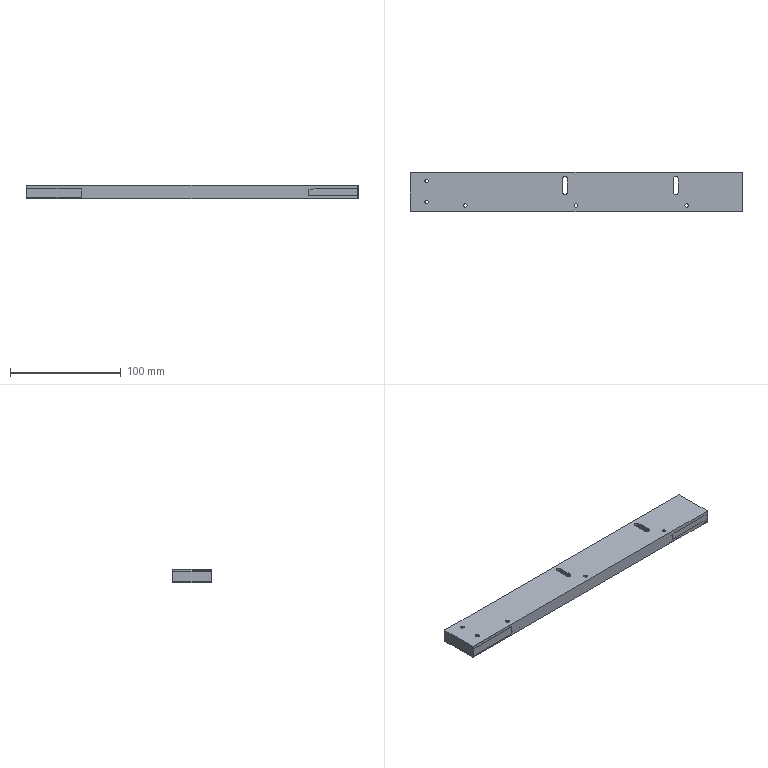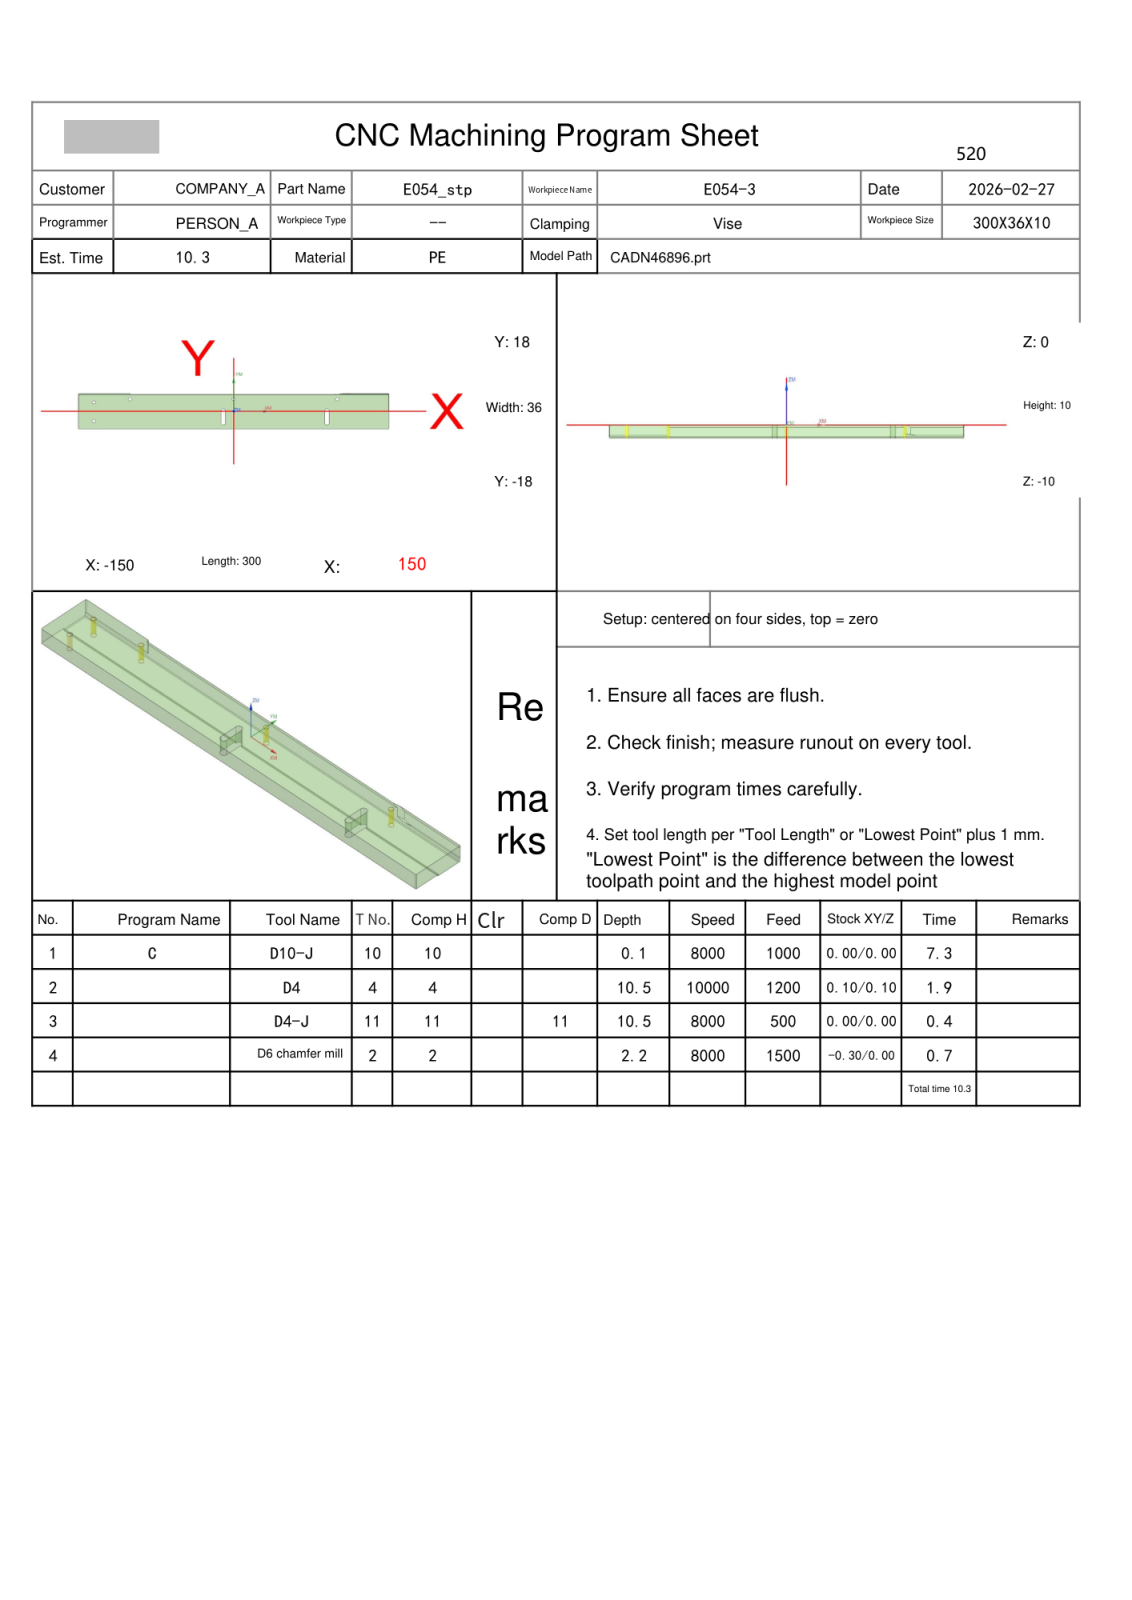NC program | NX | posted by the shop | part box 300 x 36 x 12 mm
Whole program:
%
O0001
(Machine time: 11.00 MIN)
(===Total Tool:4===)
(T10=D10-J  D=10.  R=0.   D-  H10 Z=0.    )
(T4=D4      D=4.   R=0.   D-  H04 Z=-10.5 )
(T11=D4-J   D=4.   R=0.   D11 H11 Z=-10.5 )
(T2=D6 chamfer mill   D=6.   R=0.   D-  H02 Z=-2.17 )
G80 G90 G17 G49 G40
G91 G28 Z0
M01
N1 T10 M06
(D10-J  D=10. R=0. H=10 ce=0.00 di=0.10)
G00 G90 G54 X-167. Y1.111 M03 S8000
G43 H10 Z50.
M08
Z2.55
G01 Z.55 F1000.
X-155. Y13.111
X-145.111 Y23.
X-135.222
X-155. Y3.222
Y-6.667
X-125.333 Y23.
X-115.444
X-155. Y-16.556
Y-23.
X-151.556
X-105.556 Y23.
X-95.667
X-141.667 Y-23.
X-131.778
X-85.778 Y23.
X-75.889
X-121.889 Y-23.
X-112.
X-66. Y23.
X-56.111
X-102.111 Y-23.
X-92.222
X-46.222 Y23.
X-36.333
X-82.333 Y-23.
X-72.444
X-26.444 Y23.
X-16.556
X-62.556 Y-23.
X-52.667
X-6.667 Y23.
X3.222
X-42.778 Y-23.
X-32.889
X13.111 Y23.
X23.
X-23. Y-23.
X-13.111
X32.889 Y23.
X42.778
X-3.222 Y-23.
X6.667
X52.667 Y23.
X62.556
X16.556 Y-23.
X26.444
X72.444 Y23.
X82.333
X36.333 Y-23.
X46.222
X92.222 Y23.
X102.111
X56.111 Y-23.
X66.
X112. Y23.
X121.889
X75.889 Y-23.
X85.778
X131.778 Y23.
X141.667
X95.667 Y-23.
X105.556
X151.556 Y23.
X155.
Y16.556
X115.444 Y-23.
X125.333
X155. Y6.667
Y-3.222
X135.222 Y-23.
X145.111
X155. Y-13.111
X167. Y-1.111
Z2.55
G00 Z4.
X-167. Y1.111
Z2.1
G01 Z.1
X-155. Y13.111
X-145.111 Y23.
X-135.222
X-155. Y3.222
Y-6.667
X-125.333 Y23.
X-115.444
X-155. Y-16.556
Y-23.
X-151.556
X-105.556 Y23.
X-95.667
X-141.667 Y-23.
X-131.778
X-85.778 Y23.
X-75.889
X-121.889 Y-23.
X-112.
X-66. Y23.
X-56.111
X-102.111 Y-23.
X-92.222
X-46.222 Y23.
X-36.333
X-82.333 Y-23.
X-72.444
X-26.444 Y23.
X-16.556
X-62.556 Y-23.
X-52.667
X-6.667 Y23.
X3.222
X-42.778 Y-23.
X-32.889
X13.111 Y23.
X23.
X-23. Y-23.
X-13.111
X32.889 Y23.
X42.778
X-3.222 Y-23.
X6.667
X52.667 Y23.
X62.556
X16.556 Y-23.
X26.444
X72.444 Y23.
X82.333
X36.333 Y-23.
X46.222
X92.222 Y23.
X102.111
X56.111 Y-23.
X66.
X112. Y23.
X121.889
X75.889 Y-23.
X85.778
X131.778 Y23.
X141.667
X95.667 Y-23.
X105.556
X151.556 Y23.
X155.
Y16.556
X115.444 Y-23.
X125.333
X155. Y6.667
Y-3.222
X135.222 Y-23.
X145.111
X155. Y-13.111
X167. Y-1.111
Z2.1
G00 Z50.
G00 G90 X-167. Y1.111 M03 S8000
Z50.
Z2.
G01 Z0.0 F1000.
X-155. Y13.111
X-145.111 Y23.
X-135.222
X-155. Y3.222
Y-6.667
X-125.333 Y23.
X-115.444
X-155. Y-16.556
Y-23.
X-151.556
X-105.556 Y23.
X-95.667
X-141.667 Y-23.
X-131.778
X-85.778 Y23.
X-75.889
X-121.889 Y-23.
X-112.
X-66. Y23.
X-56.111
X-102.111 Y-23.
X-92.222
X-46.222 Y23.
X-36.333
X-82.333 Y-23.
X-72.444
X-26.444 Y23.
X-16.556
X-62.556 Y-23.
X-52.667
X-6.667 Y23.
X3.222
X-42.778 Y-23.
X-32.889
X13.111 Y23.
X23.
X-23. Y-23.
X-13.111
X32.889 Y23.
X42.778
X-3.222 Y-23.
X6.667
X52.667 Y23.
X62.556
X16.556 Y-23.
X26.444
X72.444 Y23.
X82.333
X36.333 Y-23.
X46.222
X92.222 Y23.
X102.111
X56.111 Y-23.
X66.
X112. Y23.
X121.889
X75.889 Y-23.
X85.778
X131.778 Y23.
X141.667
X95.667 Y-23.
X105.556
X151.556 Y23.
X155.
Y16.556
X115.444 Y-23.
X125.333
X155. Y6.667
Y-3.222
X135.222 Y-23.
X145.111
X155. Y-13.111
X167. Y-1.111
Z2.
G00 Z50.
G91 G28 Z0.0
M05
M09
G91 G28 Z0.0
M01
N2 T04 M06
(D4  D=4. R=0. H=04 ce=0.10 di=0.10)
G00 G90 G54 X89.85 Y-5.8 M03 S10000
G43 H04 Z50.
M08
Z.5
G01 Y-11.8 Z.44 F1200.
X89.855 Y-11.867 Z.439
X89.897 Y-11.922
X89.96 Y-11.945 Z.438
X90. Y-11.95
X90.051 Y-11.952 Z.437
X90.09 Y-11.92
X90.13 Y-11.893 Z.436
X90.152 Y-11.849
X90.15 Y-11.8 Z.435
Y.2 Z.315
G03 X90. Y.35 Z.313 I-.15 J0.0
X89.85 Y.2 Z.31 I0.0 J-.15
G01 Y-11.8 Z.19
X89.855 Y-11.867 Z.189
X89.897 Y-11.922
X89.96 Y-11.945 Z.188
X90. Y-11.95
X90.051 Y-11.952 Z.187
X90.09 Y-11.92
X90.13 Y-11.893 Z.186
X90.152 Y-11.849
X90.15 Y-11.8 Z.185
Y.2 Z.065
G03 X90. Y.35 Z.063 I-.15 J0.0
X89.85 Y.2 Z.06 I0.0 J-.15
G01 Y-11.8 Z-.06
X89.855 Y-11.867 Z-.061
X89.897 Y-11.922
X89.96 Y-11.945 Z-.062
X90. Y-11.95 Z-.063
X90.051 Y-11.952
X90.09 Y-11.92
X90.13 Y-11.893 Z-.064
X90.152 Y-11.849
X90.15 Y-11.8 Z-.065
Y.2 Z-.185
G03 X90. Y.35 Z-.188 I-.15 J0.0
X89.85 Y.2 Z-.19 I0.0 J-.15
G01 Y-11.8 Z-.31
X89.855 Y-11.867 Z-.311
X89.897 Y-11.922
X89.96 Y-11.945 Z-.312
X90. Y-11.95 Z-.313
X90.051 Y-11.952
X90.09 Y-11.92
X90.13 Y-11.893 Z-.314
X90.152 Y-11.849
X90.15 Y-11.8 Z-.315
Y.2 Z-.435
G03 X90. Y.35 Z-.438 I-.15 J0.0
X89.85 Y.2 Z-.44 I0.0 J-.15
G01 Y-11.8 Z-.56
X89.855 Y-11.867 Z-.561
X89.897 Y-11.922
X89.96 Y-11.945 Z-.562
X90. Y-11.95 Z-.563
X90.051 Y-11.952
X90.09 Y-11.92
X90.13 Y-11.893 Z-.564
X90.152 Y-11.849
X90.15 Y-11.8 Z-.565
Y.2 Z-.685
G03 X90. Y.35 Z-.688 I-.15 J0.0
X89.85 Y.2 Z-.69 I0.0 J-.15
G01 Y-11.8 Z-.81
X89.855 Y-11.867 Z-.811
X89.897 Y-11.922
X89.96 Y-11.945 Z-.812
X90. Y-11.95 Z-.813
X90.051 Y-11.952
X90.09 Y-11.92
X90.13 Y-11.893 Z-.814
X90.152 Y-11.849
X90.15 Y-11.8 Z-.815
Y.2 Z-.935
G03 X90. Y.35 Z-.938 I-.15 J0.0
X89.85 Y.2 Z-.94 I0.0 J-.15
G01 Y-11.8 Z-1.06
X89.855 Y-11.867 Z-1.061
X89.897 Y-11.922
X89.96 Y-11.945 Z-1.062
X90. Y-11.95 Z-1.063
X90.051 Y-11.952
X90.09 Y-11.92
X90.13 Y-11.893 Z-1.064
X90.152 Y-11.849
X90.15 Y-11.8 Z-1.065
Y.2 Z-1.185
G03 X90. Y.35 Z-1.188 I-.15 J0.0
X89.85 Y.2 Z-1.19 I0.0 J-.15
G01 Y-11.8 Z-1.31
X89.855 Y-11.867 Z-1.311
X89.897 Y-11.922
X89.96 Y-11.945 Z-1.312
X90. Y-11.95 Z-1.313
X90.051 Y-11.952
X90.09 Y-11.92
X90.13 Y-11.893 Z-1.314
X90.152 Y-11.849
X90.15 Y-11.8 Z-1.315
Y.2 Z-1.435
G03 X90. Y.35 Z-1.438 I-.15 J0.0
X89.85 Y.2 Z-1.44 I0.0 J-.15
G01 Y-11.8 Z-1.56
X89.855 Y-11.867 Z-1.561
X89.897 Y-11.922
X89.96 Y-11.945 Z-1.562
X90. Y-11.95 Z-1.563
X90.051 Y-11.952
X90.09 Y-11.92
X90.13 Y-11.893 Z-1.564
X90.152 Y-11.849
X90.15 Y-11.8 Z-1.565
Y.2 Z-1.685
G03 X90. Y.35 Z-1.688 I-.15 J0.0
X89.85 Y.2 Z-1.69 I0.0 J-.15
G01 Y-11.8 Z-1.81
X89.855 Y-11.867 Z-1.811
X89.897 Y-11.922
X89.96 Y-11.945 Z-1.812
X90. Y-11.95 Z-1.813
X90.051 Y-11.952
X90.09 Y-11.92
X90.13 Y-11.893 Z-1.814
X90.152 Y-11.849
X90.15 Y-11.8 Z-1.815
Y.2 Z-1.935
G03 X90. Y.35 Z-1.938 I-.15 J0.0
X89.85 Y.2 Z-1.94 I0.0 J-.15
G01 Y-11.8 Z-2.06
X89.855 Y-11.867 Z-2.061
X89.897 Y-11.922
X89.96 Y-11.945 Z-2.062
X90. Y-11.95 Z-2.063
X90.051 Y-11.952
X90.09 Y-11.92
X90.13 Y-11.893 Z-2.064
X90.152 Y-11.849
X90.15 Y-11.8 Z-2.065
Y.2 Z-2.185
G03 X90. Y.35 Z-2.188 I-.15 J0.0
X89.85 Y.2 Z-2.19 I0.0 J-.15
G01 Y-11.8 Z-2.31
X89.855 Y-11.867 Z-2.311
X89.897 Y-11.922
X89.96 Y-11.945 Z-2.312
X90. Y-11.95 Z-2.313
X90.051 Y-11.952
X90.09 Y-11.92
X90.13 Y-11.893 Z-2.314
X90.152 Y-11.849
X90.15 Y-11.8 Z-2.315
Y.2 Z-2.435
G03 X90. Y.35 Z-2.438 I-.15 J0.0
X89.85 Y.2 Z-2.44 I0.0 J-.15
G01 Y-11.8 Z-2.56
X89.855 Y-11.867 Z-2.561
X89.897 Y-11.922
X89.96 Y-11.945 Z-2.562
X90. Y-11.95 Z-2.563
X90.051 Y-11.952
X90.09 Y-11.92
X90.13 Y-11.893 Z-2.564
X90.152 Y-11.849
X90.15 Y-11.8 Z-2.565
Y.2 Z-2.685
G03 X90. Y.35 Z-2.688 I-.15 J0.0
X89.85 Y.2 Z-2.69 I0.0 J-.15
G01 Y-11.8 Z-2.81
X89.855 Y-11.867 Z-2.811
X89.897 Y-11.922
X89.96 Y-11.945 Z-2.812
X90. Y-11.95 Z-2.813
X90.051 Y-11.952
X90.09 Y-11.92
X90.13 Y-11.893 Z-2.814
X90.152 Y-11.849
X90.15 Y-11.8 Z-2.815
Y.2 Z-2.935
G03 X90. Y.35 Z-2.938 I-.15 J0.0
X89.85 Y.2 Z-2.94 I0.0 J-.15
G01 Y-11.8 Z-3.06
X89.855 Y-11.867 Z-3.061
X89.897 Y-11.922
X89.96 Y-11.945 Z-3.062
X90. Y-11.95 Z-3.063
X90.051 Y-11.952
X90.09 Y-11.92
X90.13 Y-11.893 Z-3.064
X90.152 Y-11.849
X90.15 Y-11.8 Z-3.065
Y.2 Z-3.185
G03 X90. Y.35 Z-3.188 I-.15 J0.0
X89.85 Y.2 Z-3.19 I0.0 J-.15
G01 Y-11.8 Z-3.31
X89.855 Y-11.867 Z-3.311
X89.897 Y-11.922
X89.96 Y-11.945 Z-3.312
X90. Y-11.95 Z-3.313
X90.051 Y-11.952
X90.09 Y-11.92
X90.13 Y-11.893 Z-3.314
X90.152 Y-11.849
X90.15 Y-11.8 Z-3.315
Y.2 Z-3.435
G03 X90. Y.35 Z-3.438 I-.15 J0.0
X89.85 Y.2 Z-3.44 I0.0 J-.15
G01 Y-11.8 Z-3.56
X89.855 Y-11.867 Z-3.561
X89.897 Y-11.922
X89.96 Y-11.945 Z-3.562
X90. Y-11.95 Z-3.563
X90.051 Y-11.952
X90.09 Y-11.92
X90.13 Y-11.893 Z-3.564
X90.152 Y-11.849
X90.15 Y-11.8 Z-3.565
Y.2 Z-3.685
G03 X90. Y.35 Z-3.688 I-.15 J0.0
X89.85 Y.2 Z-3.69 I0.0 J-.15
G01 Y-11.8 Z-3.81
X89.855 Y-11.867 Z-3.811
X89.897 Y-11.922
X89.96 Y-11.945 Z-3.812
X90. Y-11.95 Z-3.813
X90.051 Y-11.952
X90.09 Y-11.92
X90.13 Y-11.893 Z-3.814
X90.152 Y-11.849
X90.15 Y-11.8 Z-3.815
Y.2 Z-3.935
G03 X90. Y.35 Z-3.938 I-.15 J0.0
X89.85 Y.2 Z-3.94 I0.0 J-.15
G01 Y-11.8 Z-4.06
X89.855 Y-11.867 Z-4.061
X89.897 Y-11.922
X89.96 Y-11.945 Z-4.062
X90. Y-11.95 Z-4.063
X90.051 Y-11.952
X90.09 Y-11.92
X90.13 Y-11.893 Z-4.064
X90.152 Y-11.849
X90.15 Y-11.8 Z-4.065
Y.2 Z-4.185
G03 X90. Y.35 Z-4.188 I-.15 J0.0
X89.85 Y.2 Z-4.19 I0.0 J-.15
G01 Y-11.8 Z-4.31
X89.855 Y-11.867 Z-4.311
X89.897 Y-11.922
X89.96 Y-11.945 Z-4.312
X90. Y-11.95 Z-4.313
X90.051 Y-11.952
X90.09 Y-11.92
X90.13 Y-11.893 Z-4.314
X90.152 Y-11.849
X90.15 Y-11.8 Z-4.315
Y.2 Z-4.435
G03 X90. Y.35 Z-4.438 I-.15 J0.0
X89.85 Y.2 Z-4.44 I0.0 J-.15
G01 Y-11.8 Z-4.56
X89.855 Y-11.867 Z-4.561
X89.897 Y-11.922
X89.96 Y-11.945 Z-4.562
X90. Y-11.95 Z-4.563
X90.051 Y-11.952
X90.09 Y-11.92
X90.13 Y-11.893 Z-4.564
X90.152 Y-11.849
X90.15 Y-11.8 Z-4.565
Y.2 Z-4.685
G03 X90. Y.35 Z-4.688 I-.15 J0.0
X89.85 Y.2 Z-4.69 I0.0 J-.15
G01 Y-11.8 Z-4.81
X89.855 Y-11.867 Z-4.811
X89.897 Y-11.922
X89.96 Y-11.945 Z-4.812
X90. Y-11.95 Z-4.813
X90.051 Y-11.952
X90.09 Y-11.92
X90.13 Y-11.893 Z-4.814
X90.152 Y-11.849
X90.15 Y-11.8 Z-4.815
Y.2 Z-4.935
G03 X90. Y.35 Z-4.938 I-.15 J0.0
X89.85 Y.2 Z-4.94 I0.0 J-.15
G01 Y-11.8 Z-5.06
X89.855 Y-11.867 Z-5.061
X89.897 Y-11.922
X89.96 Y-11.945 Z-5.062
X90. Y-11.95 Z-5.063
X90.051 Y-11.952
X90.09 Y-11.92
X90.13 Y-11.893 Z-5.064
X90.152 Y-11.849
X90.15 Y-11.8 Z-5.065
Y.2 Z-5.185
G03 X90. Y.35 Z-5.188 I-.15 J0.0
X89.85 Y.2 Z-5.19 I0.0 J-.15
G01 Y-11.8 Z-5.31
X89.855 Y-11.867 Z-5.311
X89.897 Y-11.922
X89.96 Y-11.945 Z-5.312
X90. Y-11.95 Z-5.313
X90.051 Y-11.952
X90.09 Y-11.92
X90.13 Y-11.893 Z-5.314
X90.152 Y-11.849
X90.15 Y-11.8 Z-5.315
Y.2 Z-5.435
G03 X90. Y.35 Z-5.438 I-.15 J0.0
X89.85 Y.2 Z-5.44 I0.0 J-.15
G01 Y-11.8 Z-5.56
X89.855 Y-11.867 Z-5.561
X89.897 Y-11.922
X89.96 Y-11.945 Z-5.562
X90. Y-11.95 Z-5.563
X90.051 Y-11.952
X90.09 Y-11.92
X90.13 Y-11.893 Z-5.564
X90.152 Y-11.849
X90.15 Y-11.8 Z-5.565
Y.2 Z-5.685
G03 X90. Y.35 Z-5.688 I-.15 J0.0
X89.85 Y.2 Z-5.69 I0.0 J-.15
G01 Y-11.8 Z-5.81
X89.855 Y-11.867 Z-5.811
X89.897 Y-11.922
X89.96 Y-11.945 Z-5.812
X90. Y-11.95 Z-5.813
X90.051 Y-11.952
X90.09 Y-11.92
X90.13 Y-11.893 Z-5.814
X90.152 Y-11.849
X90.15 Y-11.8 Z-5.815
Y.2 Z-5.935
G03 X90. Y.35 Z-5.938 I-.15 J0.0
X89.85 Y.2 Z-5.94 I0.0 J-.15
G01 Y-11.8 Z-6.06
X89.855 Y-11.867 Z-6.061
X89.897 Y-11.922
X89.96 Y-11.945 Z-6.062
X90. Y-11.95 Z-6.063
X90.051 Y-11.952
X90.09 Y-11.92
X90.13 Y-11.893 Z-6.064
X90.152 Y-11.849
X90.15 Y-11.8 Z-6.065
Y.2 Z-6.185
G03 X90. Y.35 Z-6.188 I-.15 J0.0
X89.85 Y.2 Z-6.19 I0.0 J-.15
G01 Y-11.8 Z-6.31
X89.855 Y-11.867 Z-6.311
X89.897 Y-11.922
X89.96 Y-11.945 Z-6.312
X90. Y-11.95 Z-6.313
X90.051 Y-11.952
X90.09 Y-11.92
X90.13 Y-11.893 Z-6.314
X90.152 Y-11.849
X90.15 Y-11.8 Z-6.315
Y.2 Z-6.435
G03 X90. Y.35 Z-6.438 I-.15 J0.0
X89.85 Y.2 Z-6.44 I0.0 J-.15
G01 Y-11.8 Z-6.56
X89.855 Y-11.867 Z-6.561
X89.897 Y-11.922
X89.96 Y-11.945 Z-6.562
X90. Y-11.95 Z-6.563
X90.051 Y-11.952
X90.09 Y-11.92
X90.13 Y-11.893 Z-6.564
X90.152 Y-11.849
X90.15 Y-11.8 Z-6.565
Y.2 Z-6.685
G03 X90. Y.35 Z-6.688 I-.15 J0.0
X89.85 Y.2 Z-6.69 I0.0 J-.15
G01 Y-11.8 Z-6.81
X89.855 Y-11.867 Z-6.811
X89.897 Y-11.922
X89.96 Y-11.945 Z-6.812
X90. Y-11.95 Z-6.813
X90.051 Y-11.952
X90.09 Y-11.92
X90.13 Y-11.893 Z-6.814
X90.152 Y-11.849
X90.15 Y-11.8 Z-6.815
Y.2 Z-6.935
G03 X90. Y.35 Z-6.938 I-.15 J0.0
X89.85 Y.2 Z-6.94 I0.0 J-.15
G01 Y-11.8 Z-7.06
X89.855 Y-11.867 Z-7.061
X89.897 Y-11.922
X89.96 Y-11.945 Z-7.062
X90. Y-11.95 Z-7.063
X90.051 Y-11.952
X90.09 Y-11.92
X90.13 Y-11.893 Z-7.064
X90.152 Y-11.849
X90.15 Y-11.8 Z-7.065
Y.2 Z-7.185
G03 X90. Y.35 Z-7.188 I-.15 J0.0
X89.85 Y.2 Z-7.19 I0.0 J-.15
G01 Y-11.8 Z-7.31
X89.855 Y-11.867 Z-7.311
X89.897 Y-11.922
X89.96 Y-11.945 Z-7.312
X90. Y-11.95 Z-7.313
X90.051 Y-11.952
X90.09 Y-11.92
X90.13 Y-11.893 Z-7.314
X90.152 Y-11.849
X90.15 Y-11.8 Z-7.315
Y.2 Z-7.435
G03 X90. Y.35 Z-7.438 I-.15 J0.0
X89.85 Y.2 Z-7.44 I0.0 J-.15
G01 Y-11.8 Z-7.56
X89.855 Y-11.867 Z-7.561
X89.897 Y-11.922
X89.96 Y-11.945 Z-7.562
X90. Y-11.95 Z-7.563
X90.051 Y-11.952
X90.09 Y-11.92
X90.13 Y-11.893 Z-7.564
X90.152 Y-11.849
X90.15 Y-11.8 Z-7.565
Y.2 Z-7.685
G03 X90. Y.35 Z-7.688 I-.15 J0.0
X89.85 Y.2 Z-7.69 I0.0 J-.15
G01 Y-11.8 Z-7.81
X89.855 Y-11.867 Z-7.811
X89.897 Y-11.922
X89.96 Y-11.945 Z-7.812
X90. Y-11.95 Z-7.813
X90.051 Y-11.952
X90.09 Y-11.92
X90.13 Y-11.893 Z-7.814
X90.152 Y-11.849
X90.15 Y-11.8 Z-7.815
Y.2 Z-7.935
G03 X90. Y.35 Z-7.938 I-.15 J0.0
X89.85 Y.2 Z-7.94 I0.0 J-.15
G01 Y-11.8 Z-8.06
X89.855 Y-11.867 Z-8.061
X89.897 Y-11.922
X89.96 Y-11.945 Z-8.062
X90. Y-11.95 Z-8.063
X90.051 Y-11.952
X90.09 Y-11.92
X90.13 Y-11.893 Z-8.064
X90.152 Y-11.849
X90.15 Y-11.8 Z-8.065
Y.2 Z-8.185
G03 X90. Y.35 Z-8.188 I-.15 J0.0
X89.85 Y.2 Z-8.19 I0.0 J-.15
G01 Y-11.8 Z-8.31
X89.855 Y-11.867 Z-8.311
X89.897 Y-11.922
X89.96 Y-11.945 Z-8.312
X90. Y-11.95 Z-8.313
X90.051 Y-11.952
X90.09 Y-11.92
X90.13 Y-11.893 Z-8.314
X90.152 Y-11.849
X90.15 Y-11.8 Z-8.315
Y.2 Z-8.435
G03 X90. Y.35 Z-8.438 I-.15 J0.0
X89.85 Y.2 Z-8.44 I0.0 J-.15
G01 Y-11.8 Z-8.56
X89.855 Y-11.867 Z-8.561
X89.897 Y-11.922
X89.96 Y-11.945 Z-8.562
X90. Y-11.95 Z-8.563
X90.051 Y-11.952
X90.09 Y-11.92
X90.13 Y-11.893 Z-8.564
X90.152 Y-11.849
X90.15 Y-11.8 Z-8.565
Y.2 Z-8.685
G03 X90. Y.35 Z-8.688 I-.15 J0.0
X89.85 Y.2 Z-8.69 I0.0 J-.15
G01 Y-11.8 Z-8.81
X89.855 Y-11.867 Z-8.811
X89.897 Y-11.922
X89.96 Y-11.945 Z-8.812
X90. Y-11.95 Z-8.813
X90.051 Y-11.952
X90.09 Y-11.92
X90.13 Y-11.893 Z-8.814
X90.152 Y-11.849
X90.15 Y-11.8 Z-8.815
Y.2 Z-8.935
G03 X90. Y.35 Z-8.938 I-.15 J0.0
X89.85 Y.2 Z-8.94 I0.0 J-.15
G01 Y-11.8 Z-9.06
X89.855 Y-11.867 Z-9.061
X89.897 Y-11.922
X89.96 Y-11.945 Z-9.062
X90. Y-11.95 Z-9.063
X90.051 Y-11.952
X90.09 Y-11.92
X90.13 Y-11.893 Z-9.064
X90.152 Y-11.849
X90.15 Y-11.8 Z-9.065
Y.2 Z-9.185
G03 X90. Y.35 Z-9.188 I-.15 J0.0
X89.85 Y.2 Z-9.19 I0.0 J-.15
G01 Y-11.8 Z-9.31
X89.855 Y-11.867 Z-9.311
X89.897 Y-11.922
X89.96 Y-11.945 Z-9.312
X90. Y-11.95 Z-9.313
X90.051 Y-11.952
X90.09 Y-11.92
X90.13 Y-11.893 Z-9.314
X90.152 Y-11.849
X90.15 Y-11.8 Z-9.315
Y.2 Z-9.435
G03 X90. Y.35 Z-9.438 I-.15 J0.0
X89.85 Y.2 Z-9.44 I0.0 J-.15
G01 Y-11.8 Z-9.56
X89.855 Y-11.867 Z-9.561
X89.897 Y-11.922
X89.96 Y-11.945 Z-9.562
X90. Y-11.95 Z-9.563
X90.051 Y-11.952
X90.09 Y-11.92
X90.13 Y-11.893 Z-9.564
X90.152 Y-11.849
X90.15 Y-11.8 Z-9.565
Y.2 Z-9.685
G03 X90. Y.35 Z-9.688 I-.15 J0.0
X89.85 Y.2 Z-9.69 I0.0 J-.15
G01 Y-11.8 Z-9.81
X89.855 Y-11.867 Z-9.811
X89.897 Y-11.922
X89.96 Y-11.945 Z-9.812
X90. Y-11.95 Z-9.813
X90.051 Y-11.952
X90.09 Y-11.92
X90.13 Y-11.893 Z-9.814
X90.152 Y-11.849
X90.15 Y-11.8 Z-9.815
Y.2 Z-9.935
G03 X90. Y.35 Z-9.938 I-.15 J0.0
X89.85 Y.2 Z-9.94 I0.0 J-.15
G01 Y-11.8 Z-10.06
X89.855 Y-11.867 Z-10.061
X89.897 Y-11.922
X89.96 Y-11.945 Z-10.062
X90. Y-11.95 Z-10.063
X90.051 Y-11.952
X90.09 Y-11.92
X90.13 Y-11.893 Z-10.064
X90.152 Y-11.849
X90.15 Y-11.8 Z-10.065
Y.2 Z-10.185
G03 X90. Y.35 Z-10.188 I-.15 J0.0
X89.85 Y.2 Z-10.19 I0.0 J-.15
G01 Y-11.8 Z-10.31
X89.855 Y-11.867 Z-10.311
X89.897 Y-11.922
X89.96 Y-11.945 Z-10.312
X90. Y-11.95 Z-10.313
X90.051 Y-11.952
X90.09 Y-11.92
X90.13 Y-11.893 Z-10.314
X90.152 Y-11.849
X90.15 Y-11.8 Z-10.315
Y.2 Z-10.435
G03 X90. Y.35 Z-10.438 I-.15 J0.0
X89.85 Y.2 Z-10.44 I0.0 J-.15
G01 Y-5.8 Z-10.5
Y-11.8
G03 X90. Y-11.95 I.15 J0.0
X90.15 Y-11.8 I0.0 J.15
G01 Y.2
G03 X90. Y.35 I-.15 J0.0
X89.85 Y.2 I0.0 J-.15
G01 Y-5.8
Y-6.3
Z-9.5
G00 Z50.
X-9.85 Y-5.8
Z.5
G01 Y.2 Z.44
X-9.848 Y.249 Z.439
X-9.87 Y.293
X-9.91 Y.32 Z.438
X-9.949 Y.352
X-10. Y.35
G03 X-10.15 Y.2 Z.435 I0.0 J-.15
G01 Y-11.8 Z.315
G03 X-10. Y-11.95 Z.313 I.15 J0.0
X-9.85 Y-11.8 Z.31 I0.0 J.15
G01 Y.2 Z.19
X-9.848 Y.249 Z.189
X-9.87 Y.293
X-9.91 Y.32 Z.188
X-9.949 Y.352
X-10. Y.35
G03 X-10.15 Y.2 Z.185 I0.0 J-.15
G01 Y-11.8 Z.065
G03 X-10. Y-11.95 Z.063 I.15 J0.0
X-9.85 Y-11.8 Z.06 I0.0 J.15
G01 Y.2 Z-.06
X-9.848 Y.249 Z-.061
X-9.87 Y.293
X-9.91 Y.32 Z-.062
X-9.949 Y.352
X-10. Y.35 Z-.063
G03 X-10.15 Y.2 Z-.065 I0.0 J-.15
G01 Y-11.8 Z-.185
G03 X-10. Y-11.95 Z-.188 I.15 J0.0
X-9.85 Y-11.8 Z-.19 I0.0 J.15
G01 Y.2 Z-.31
X-9.848 Y.249 Z-.311
X-9.87 Y.293
X-9.91 Y.32 Z-.312
X-9.949 Y.352
X-10. Y.35 Z-.313
G03 X-10.15 Y.2 Z-.315 I0.0 J-.15
G01 Y-11.8 Z-.435
G03 X-10. Y-11.95 Z-.438 I.15 J0.0
X-9.85 Y-11.8 Z-.44 I0.0 J.15
G01 Y.2 Z-.56
X-9.848 Y.249 Z-.561
X-9.87 Y.293
X-9.91 Y.32 Z-.562
X-9.949 Y.352
X-10. Y.35 Z-.563
G03 X-10.15 Y.2 Z-.565 I0.0 J-.15
G01 Y-11.8 Z-.685
G03 X-10. Y-11.95 Z-.688 I.15 J0.0
X-9.85 Y-11.8 Z-.69 I0.0 J.15
G01 Y.2 Z-.81
X-9.848 Y.249 Z-.811
X-9.87 Y.293
X-9.91 Y.32 Z-.812
X-9.949 Y.352
X-10. Y.35 Z-.813
G03 X-10.15 Y.2 Z-.815 I0.0 J-.15
G01 Y-11.8 Z-.935
G03 X-10. Y-11.95 Z-.938 I.15 J0.0
X-9.85 Y-11.8 Z-.94 I0.0 J.15
G01 Y.2 Z-1.06
X-9.848 Y.249 Z-1.061
X-9.87 Y.293
X-9.91 Y.32 Z-1.062
X-9.949 Y.352
X-10. Y.35 Z-1.063
G03 X-10.15 Y.2 Z-1.065 I0.0 J-.15
G01 Y-11.8 Z-1.185
G03 X-10. Y-11.95 Z-1.188 I.15 J0.0
X-9.85 Y-11.8 Z-1.19 I0.0 J.15
G01 Y.2 Z-1.31
X-9.848 Y.249 Z-1.311
X-9.87 Y.293
X-9.91 Y.32 Z-1.312
X-9.949 Y.352
X-10. Y.35 Z-1.313
G03 X-10.15 Y.2 Z-1.315 I0.0 J-.15
G01 Y-11.8 Z-1.435
G03 X-10. Y-11.95 Z-1.438 I.15 J0.0
X-9.85 Y-11.8 Z-1.44 I0.0 J.15
G01 Y.2 Z-1.56
X-9.848 Y.249 Z-1.561
X-9.87 Y.293
X-9.91 Y.32 Z-1.562
X-9.949 Y.352
X-10. Y.35 Z-1.563
G03 X-10.15 Y.2 Z-1.565 I0.0 J-.15
G01 Y-11.8 Z-1.685
G03 X-10. Y-11.95 Z-1.688 I.15 J0.0
X-9.85 Y-11.8 Z-1.69 I0.0 J.15
G01 Y.2 Z-1.81
X-9.848 Y.249 Z-1.811
X-9.87 Y.293
X-9.91 Y.32 Z-1.812
X-9.949 Y.352
X-10. Y.35 Z-1.813
G03 X-10.15 Y.2 Z-1.815 I0.0 J-.15
G01 Y-11.8 Z-1.935
G03 X-10. Y-11.95 Z-1.938 I.15 J0.0
X-9.85 Y-11.8 Z-1.94 I0.0 J.15
G01 Y.2 Z-2.06
X-9.848 Y.249 Z-2.061
X-9.87 Y.293
X-9.91 Y.32 Z-2.062
X-9.949 Y.352
X-10. Y.35 Z-2.063
G03 X-10.15 Y.2 Z-2.065 I0.0 J-.15
G01 Y-11.8 Z-2.185
G03 X-10. Y-11.95 Z-2.188 I.15 J0.0
X-9.85 Y-11.8 Z-2.19 I0.0 J.15
G01 Y.2 Z-2.31
X-9.848 Y.249 Z-2.311
X-9.87 Y.293
X-9.91 Y.32 Z-2.312
X-9.949 Y.352
X-10. Y.35 Z-2.313
G03 X-10.15 Y.2 Z-2.315 I0.0 J-.15
G01 Y-11.8 Z-2.435
G03 X-10. Y-11.95 Z-2.438 I.15 J0.0
X-9.85 Y-11.8 Z-2.44 I0.0 J.15
G01 Y.2 Z-2.56
X-9.848 Y.249 Z-2.561
X-9.87 Y.293
X-9.91 Y.32 Z-2.562
X-9.949 Y.352
X-10. Y.35 Z-2.563
G03 X-10.15 Y.2 Z-2.565 I0.0 J-.15
G01 Y-11.8 Z-2.685
G03 X-10. Y-11.95 Z-2.688 I.15 J0.0
X-9.85 Y-11.8 Z-2.69 I0.0 J.15
G01 Y.2 Z-2.81
X-9.848 Y.249 Z-2.811
X-9.87 Y.293
X-9.91 Y.32 Z-2.812
X-9.949 Y.352
X-10. Y.35 Z-2.813
G03 X-10.15 Y.2 Z-2.815 I0.0 J-.15
G01 Y-11.8 Z-2.935
G03 X-10. Y-11.95 Z-2.938 I.15 J0.0
X-9.85 Y-11.8 Z-2.94 I0.0 J.15
G01 Y.2 Z-3.06
X-9.848 Y.249 Z-3.061
X-9.87 Y.293
X-9.91 Y.32 Z-3.062
X-9.949 Y.352
X-10. Y.35 Z-3.063
G03 X-10.15 Y.2 Z-3.065 I0.0 J-.15
G01 Y-11.8 Z-3.185
G03 X-10. Y-11.95 Z-3.188 I.15 J0.0
X-9.85 Y-11.8 Z-3.19 I0.0 J.15
G01 Y.2 Z-3.31
X-9.848 Y.249 Z-3.311
X-9.87 Y.293
X-9.91 Y.32 Z-3.312
X-9.949 Y.352
X-10. Y.35 Z-3.313
G03 X-10.15 Y.2 Z-3.315 I0.0 J-.15
G01 Y-11.8 Z-3.435
G03 X-10. Y-11.95 Z-3.438 I.15 J0.0
X-9.85 Y-11.8 Z-3.44 I0.0 J.15
G01 Y.2 Z-3.56
X-9.848 Y.249 Z-3.561
X-9.87 Y.293
X-9.91 Y.32 Z-3.562
X-9.949 Y.352
X-10. Y.35 Z-3.563
G03 X-10.15 Y.2 Z-3.565 I0.0 J-.15
G01 Y-11.8 Z-3.685
G03 X-10. Y-11.95 Z-3.688 I.15 J0.0
X-9.85 Y-11.8 Z-3.69 I0.0 J.15
G01 Y.2 Z-3.81
X-9.848 Y.249 Z-3.811
X-9.87 Y.293
X-9.91 Y.32 Z-3.812
X-9.949 Y.352
X-10. Y.35 Z-3.813
G03 X-10.15 Y.2 Z-3.815 I0.0 J-.15
G01 Y-11.8 Z-3.935
G03 X-10. Y-11.95 Z-3.938 I.15 J0.0
X-9.85 Y-11.8 Z-3.94 I0.0 J.15
G01 Y.2 Z-4.06
X-9.848 Y.249 Z-4.061
X-9.87 Y.293
X-9.91 Y.32 Z-4.062
X-9.949 Y.352
X-10. Y.35 Z-4.063
G03 X-10.15 Y.2 Z-4.065 I0.0 J-.15
G01 Y-11.8 Z-4.185
G03 X-10. Y-11.95 Z-4.188 I.15 J0.0
X-9.85 Y-11.8 Z-4.19 I0.0 J.15
G01 Y.2 Z-4.31
X-9.848 Y.249 Z-4.311
X-9.87 Y.293
X-9.91 Y.32 Z-4.312
X-9.949 Y.352
X-10. Y.35 Z-4.313
G03 X-10.15 Y.2 Z-4.315 I0.0 J-.15
G01 Y-11.8 Z-4.435
G03 X-10. Y-11.95 Z-4.438 I.15 J0.0
X-9.85 Y-11.8 Z-4.44 I0.0 J.15
G01 Y.2 Z-4.56
X-9.848 Y.249 Z-4.561
X-9.87 Y.293
X-9.91 Y.32 Z-4.562
X-9.949 Y.352
X-10. Y.35 Z-4.563
G03 X-10.15 Y.2 Z-4.565 I0.0 J-.15
G01 Y-11.8 Z-4.685
G03 X-10. Y-11.95 Z-4.688 I.15 J0.0
X-9.85 Y-11.8 Z-4.69 I0.0 J.15
G01 Y.2 Z-4.81
X-9.848 Y.249 Z-4.811
X-9.87 Y.293
X-9.91 Y.32 Z-4.812
X-9.949 Y.352
X-10. Y.35 Z-4.813
G03 X-10.15 Y.2 Z-4.815 I0.0 J-.15
G01 Y-11.8 Z-4.935
G03 X-10. Y-11.95 Z-4.938 I.15 J0.0
X-9.85 Y-11.8 Z-4.94 I0.0 J.15
G01 Y.2 Z-5.06
X-9.848 Y.249 Z-5.061
X-9.87 Y.293
X-9.91 Y.32 Z-5.062
X-9.949 Y.352
X-10. Y.35 Z-5.063
G03 X-10.15 Y.2 Z-5.065 I0.0 J-.15
G01 Y-11.8 Z-5.185
G03 X-10. Y-11.95 Z-5.188 I.15 J0.0
X-9.85 Y-11.8 Z-5.19 I0.0 J.15
G01 Y.2 Z-5.31
X-9.848 Y.249 Z-5.311
X-9.87 Y.293
X-9.91 Y.32 Z-5.312
X-9.949 Y.352
X-10. Y.35 Z-5.313
G03 X-10.15 Y.2 Z-5.315 I0.0 J-.15
G01 Y-11.8 Z-5.435
G03 X-10. Y-11.95 Z-5.438 I.15 J0.0
X-9.85 Y-11.8 Z-5.44 I0.0 J.15
G01 Y.2 Z-5.56
X-9.848 Y.249 Z-5.561
X-9.87 Y.293
X-9.91 Y.32 Z-5.562
X-9.949 Y.352
X-10. Y.35 Z-5.563
G03 X-10.15 Y.2 Z-5.565 I0.0 J-.15
G01 Y-11.8 Z-5.685
G03 X-10. Y-11.95 Z-5.688 I.15 J0.0
X-9.85 Y-11.8 Z-5.69 I0.0 J.15
G01 Y.2 Z-5.81
X-9.848 Y.249 Z-5.811
X-9.87 Y.293
X-9.91 Y.32 Z-5.812
X-9.949 Y.352
X-10. Y.35 Z-5.813
G03 X-10.15 Y.2 Z-5.815 I0.0 J-.15
G01 Y-11.8 Z-5.935
G03 X-10. Y-11.95 Z-5.938 I.15 J0.0
X-9.85 Y-11.8 Z-5.94 I0.0 J.15
G01 Y.2 Z-6.06
X-9.848 Y.249 Z-6.061
X-9.87 Y.293
X-9.91 Y.32 Z-6.062
X-9.949 Y.352
X-10. Y.35 Z-6.063
G03 X-10.15 Y.2 Z-6.065 I0.0 J-.15
G01 Y-11.8 Z-6.185
G03 X-10. Y-11.95 Z-6.188 I.15 J0.0
X-9.85 Y-11.8 Z-6.19 I0.0 J.15
G01 Y.2 Z-6.31
X-9.848 Y.249 Z-6.311
X-9.87 Y.293
X-9.91 Y.32 Z-6.312
X-9.949 Y.352
X-10. Y.35 Z-6.313
G03 X-10.15 Y.2 Z-6.315 I0.0 J-.15
G01 Y-11.8 Z-6.435
G03 X-10. Y-11.95 Z-6.438 I.15 J0.0
X-9.85 Y-11.8 Z-6.44 I0.0 J.15
G01 Y.2 Z-6.56
X-9.848 Y.249 Z-6.561
X-9.87 Y.293
X-9.91 Y.32 Z-6.562
X-9.949 Y.352
X-10. Y.35 Z-6.563
G03 X-10.15 Y.2 Z-6.565 I0.0 J-.15
G01 Y-11.8 Z-6.685
G03 X-10. Y-11.95 Z-6.688 I.15 J0.0
X-9.85 Y-11.8 Z-6.69 I0.0 J.15
G01 Y.2 Z-6.81
X-9.848 Y.249 Z-6.811
X-9.87 Y.293
X-9.91 Y.32 Z-6.812
X-9.949 Y.352
X-10. Y.35 Z-6.813
G03 X-10.15 Y.2 Z-6.815 I0.0 J-.15
G01 Y-11.8 Z-6.935
G03 X-10. Y-11.95 Z-6.938 I.15 J0.0
X-9.85 Y-11.8 Z-6.94 I0.0 J.15
G01 Y.2 Z-7.06
X-9.848 Y.249 Z-7.061
X-9.87 Y.293
X-9.91 Y.32 Z-7.062
X-9.949 Y.352
X-10. Y.35 Z-7.063
G03 X-10.15 Y.2 Z-7.065 I0.0 J-.15
G01 Y-11.8 Z-7.185
G03 X-10. Y-11.95 Z-7.188 I.15 J0.0
X-9.85 Y-11.8 Z-7.19 I0.0 J.15
G01 Y.2 Z-7.31
X-9.848 Y.249 Z-7.311
X-9.87 Y.293
X-9.91 Y.32 Z-7.312
X-9.949 Y.352
X-10. Y.35 Z-7.313
G03 X-10.15 Y.2 Z-7.315 I0.0 J-.15
G01 Y-11.8 Z-7.435
G03 X-10. Y-11.95 Z-7.438 I.15 J0.0
X-9.85 Y-11.8 Z-7.44 I0.0 J.15
G01 Y.2 Z-7.56
X-9.848 Y.249 Z-7.561
X-9.87 Y.293
X-9.91 Y.32 Z-7.562
X-9.949 Y.352
X-10. Y.35 Z-7.563
G03 X-10.15 Y.2 Z-7.565 I0.0 J-.15
G01 Y-11.8 Z-7.685
G03 X-10. Y-11.95 Z-7.688 I.15 J0.0
X-9.85 Y-11.8 Z-7.69 I0.0 J.15
G01 Y.2 Z-7.81
X-9.848 Y.249 Z-7.811
X-9.87 Y.293
X-9.91 Y.32 Z-7.812
X-9.949 Y.352
X-10. Y.35 Z-7.813
G03 X-10.15 Y.2 Z-7.815 I0.0 J-.15
G01 Y-11.8 Z-7.935
G03 X-10. Y-11.95 Z-7.938 I.15 J0.0
X-9.85 Y-11.8 Z-7.94 I0.0 J.15
G01 Y.2 Z-8.06
X-9.848 Y.249 Z-8.061
X-9.87 Y.293
X-9.91 Y.32 Z-8.062
X-9.949 Y.352
X-10. Y.35 Z-8.063
G03 X-10.15 Y.2 Z-8.065 I0.0 J-.15
G01 Y-11.8 Z-8.185
G03 X-10. Y-11.95 Z-8.188 I.15 J0.0
X-9.85 Y-11.8 Z-8.19 I0.0 J.15
G01 Y.2 Z-8.31
X-9.848 Y.249 Z-8.311
X-9.87 Y.293
X-9.91 Y.32 Z-8.312
X-9.949 Y.352
X-10. Y.35 Z-8.313
G03 X-10.15 Y.2 Z-8.315 I0.0 J-.15
G01 Y-11.8 Z-8.435
G03 X-10. Y-11.95 Z-8.438 I.15 J0.0
X-9.85 Y-11.8 Z-8.44 I0.0 J.15
G01 Y.2 Z-8.56
X-9.848 Y.249 Z-8.561
X-9.87 Y.293
X-9.91 Y.32 Z-8.562
X-9.949 Y.352
X-10. Y.35 Z-8.563
G03 X-10.15 Y.2 Z-8.565 I0.0 J-.15
G01 Y-11.8 Z-8.685
G03 X-10. Y-11.95 Z-8.688 I.15 J0.0
X-9.85 Y-11.8 Z-8.69 I0.0 J.15
G01 Y.2 Z-8.81
X-9.848 Y.249 Z-8.811
X-9.87 Y.293
X-9.91 Y.32 Z-8.812
X-9.949 Y.352
X-10. Y.35 Z-8.813
G03 X-10.15 Y.2 Z-8.815 I0.0 J-.15
G01 Y-11.8 Z-8.935
G03 X-10. Y-11.95 Z-8.938 I.15 J0.0
X-9.85 Y-11.8 Z-8.94 I0.0 J.15
G01 Y.2 Z-9.06
X-9.848 Y.249 Z-9.061
X-9.87 Y.293
X-9.91 Y.32 Z-9.062
X-9.949 Y.352
X-10. Y.35 Z-9.063
G03 X-10.15 Y.2 Z-9.065 I0.0 J-.15
G01 Y-11.8 Z-9.185
G03 X-10. Y-11.95 Z-9.188 I.15 J0.0
X-9.85 Y-11.8 Z-9.19 I0.0 J.15
G01 Y.2 Z-9.31
X-9.848 Y.249 Z-9.311
X-9.87 Y.293
X-9.91 Y.32 Z-9.312
X-9.949 Y.352
X-10. Y.35 Z-9.313
G03 X-10.15 Y.2 Z-9.315 I0.0 J-.15
G01 Y-11.8 Z-9.435
G03 X-10. Y-11.95 Z-9.438 I.15 J0.0
X-9.85 Y-11.8 Z-9.44 I0.0 J.15
G01 Y.2 Z-9.56
X-9.848 Y.249 Z-9.561
X-9.87 Y.293
X-9.91 Y.32 Z-9.562
X-9.949 Y.352
X-10. Y.35 Z-9.563
G03 X-10.15 Y.2 Z-9.565 I0.0 J-.15
G01 Y-11.8 Z-9.685
G03 X-10. Y-11.95 Z-9.688 I.15 J0.0
X-9.85 Y-11.8 Z-9.69 I0.0 J.15
G01 Y.2 Z-9.81
X-9.848 Y.249 Z-9.811
X-9.87 Y.293
X-9.91 Y.32 Z-9.812
X-9.949 Y.352
X-10. Y.35 Z-9.813
G03 X-10.15 Y.2 Z-9.815 I0.0 J-.15
G01 Y-11.8 Z-9.935
G03 X-10. Y-11.95 Z-9.938 I.15 J0.0
X-9.85 Y-11.8 Z-9.94 I0.0 J.15
G01 Y.2 Z-10.06
X-9.848 Y.249 Z-10.061
X-9.87 Y.293
X-9.91 Y.32 Z-10.062
X-9.949 Y.352
X-10. Y.35 Z-10.063
G03 X-10.15 Y.2 Z-10.065 I0.0 J-.15
G01 Y-11.8 Z-10.185
G03 X-10. Y-11.95 Z-10.188 I.15 J0.0
X-9.85 Y-11.8 Z-10.19 I0.0 J.15
G01 Y.2 Z-10.31
X-9.848 Y.249 Z-10.311
X-9.87 Y.293
X-9.91 Y.32 Z-10.312
X-9.949 Y.352
X-10. Y.35 Z-10.313
G03 X-10.15 Y.2 Z-10.315 I0.0 J-.15
G01 Y-11.8 Z-10.435
G03 X-10. Y-11.95 Z-10.438 I.15 J0.0
X-9.85 Y-11.8 Z-10.44 I0.0 J.15
G01 Y-5.8 Z-10.5
Y.2
G03 X-10. Y.35 I-.15 J0.0
X-10.15 Y.2 I0.0 J-.15
G01 Y-11.8
G03 X-10. Y-11.95 I.15 J0.0
X-9.85 Y-11.8 I0.0 J.15
G01 Y-5.8
Y-5.3
Z-9.5
G00 Z50.
G91 G28 Z0.0
M05
M09
G91 G28 Z0.0
M01
N3 T11 M06
(D4-J  D=4. R=0. H=11 ce=0.00 di=0.00)
G00 G90 G54 X90. Y-6. M03 S8000
G43 H11 Z50.
M08
Z-3.
G01 Z-3.5 F500.
G41 D11
X90.05
G03 X90.25 Y-5.8 I0.0 J.2
G01 Y.2
G03 X90. Y.45 I-.25 J0.0
X89.75 Y.2 I0.0 J-.25
G01 Y-11.8
G03 X90. Y-12.05 I.25 J0.0
X90.25 Y-11.8 I0.0 J.25
G01 Y-5.8
Y-5.3
G03 X90.05 Y-5.1 I-.2 J0.0
G01 G40 X90.
Z-3.
G00 Z1.
Y-6.
Z-6.5
G01 Z-7.
G41 D11
X90.05
G03 X90.25 Y-5.8 I0.0 J.2
G01 Y.2
G03 X90. Y.45 I-.25 J0.0
X89.75 Y.2 I0.0 J-.25
G01 Y-11.8
G03 X90. Y-12.05 I.25 J0.0
X90.25 Y-11.8 I0.0 J.25
G01 Y-5.8
Y-5.3
G03 X90.05 Y-5.1 I-.2 J0.0
G01 G40 X90.
Z-6.5
G00 Z-2.5
Y-6.
Z-10.
G01 Z-10.5
G41 D11
X90.05
G03 X90.25 Y-5.8 I0.0 J.2
G01 Y.2
G03 X90. Y.45 I-.25 J0.0
X89.75 Y.2 I0.0 J-.25
G01 Y-11.8
G03 X90. Y-12.05 I.25 J0.0
X90.25 Y-11.8 I0.0 J.25
G01 Y-5.8
Y-5.3
G03 X90.05 Y-5.1 I-.2 J0.0
G01 G40 X90.
Z-10.
G00 Z50.
X-10. Y-6.
Z-3.
G01 Z-3.5
G41 D11
X-9.95
G03 X-9.75 Y-5.8 I0.0 J.2
G01 Y.2
G03 X-10. Y.45 I-.25 J0.0
X-10.25 Y.2 I0.0 J-.25
G01 Y-11.8
G03 X-10. Y-12.05 I.25 J0.0
X-9.75 Y-11.8 I0.0 J.25
G01 Y-5.8
Y-5.3
G03 X-9.95 Y-5.1 I-.2 J0.0
G01 G40 X-10.
Z-3.
G00 Z1.
Y-6.
Z-6.5
G01 Z-7.
G41 D11
X-9.95
G03 X-9.75 Y-5.8 I0.0 J.2
G01 Y.2
G03 X-10. Y.45 I-.25 J0.0
X-10.25 Y.2 I0.0 J-.25
G01 Y-11.8
G03 X-10. Y-12.05 I.25 J0.0
X-9.75 Y-11.8 I0.0 J.25
G01 Y-5.8
Y-5.3
G03 X-9.95 Y-5.1 I-.2 J0.0
G01 G40 X-10.
Z-6.5
G00 Z-2.5
Y-6.
Z-10.
G01 Z-10.5
G41 D11
X-9.95
G03 X-9.75 Y-5.8 I0.0 J.2
G01 Y.2
G03 X-10. Y.45 I-.25 J0.0
X-10.25 Y.2 I0.0 J-.25
G01 Y-11.8
G03 X-10. Y-12.05 I.25 J0.0
X-9.75 Y-11.8 I0.0 J.25
G01 Y-5.8
Y-5.3
G03 X-9.95 Y-5.1 I-.2 J0.0
G01 G40 X-10.
Z-10.
G00 Z50.
G91 G28 Z0.0
M05
M09
G91 G28 Z0.0
M01
N4 T02 M06
(D6 chamfer mill  D=6. R=0. H=02 ce=0.00 di=0.00)
G00 G90 G54 X100. Y12.2 M03 S8000
G43 H02 Z50.
M08
G98 G81 X100. Y12.2 Z-2.171 R3. F1000.
X0.0
X-100.
X-135. Y9.
Y-10.
G80
G00 Z50.
G00 G90 X91.55 Y-4.542 M03 S7000
Z50.
Z2.5
G01 Y.296 Z.739 F1500.
X91.515 Y.543 Z.648
X91.44 Y.781 Z.557
X91.329 Y1.004 Z.467
X91.183 Y1.206 Z.376
X91.006 Y1.383 Z.285
X90.804 Y1.529 Z.194
X90.581 Y1.64 Z.104
X90.343 Y1.715 Z.013
X90.096 Y1.75 Z-.078
X89.904 Z-.148
X89.657 Y1.715 Z-.239
X89.419 Y1.64 Z-.33
X89.196 Y1.529 Z-.42
X88.994 Y1.383 Z-.511
X88.817 Y1.206 Z-.602
X88.671 Y1.004 Z-.693
X88.56 Y.781 Z-.783
X88.485 Y.543 Z-.874
X88.45 Y.296 Z-.965
Y.2 Z-1.
Y-11.8
G03 X90. Y-13.35 I1.55 J0.0
X91.55 Y-11.8 I0.0 J1.55
G01 Y.2
G03 X90. Y1.75 I-1.55 J0.0
X88.45 Y.2 I0.0 J-1.55
G01 Y-.3
Z1.5
G00 Z50.
X-140.546 Y-18.7
Z2.5
G01 X-149.376 Z-.714
X-149.453 Z-.742
X-149.66 Y-18.662 Z-.819
X-149.855 Y-18.581 Z-.895
X-150.028 Y-18.462 Z-.972
X-150.083 Y-18.407 Z-1.
X-150.407 Y-18.083
G02 X-150.7 Y-17.376 I.707 J.707
G01 Y17.376
G02 X-150.407 Y18.083 I1. J0.0
G01 X-150.083 Y18.407
G02 X-149.376 Y18.7 I.707 J-.707
G01 X-149.374
X101.876 Y18.2
X149.7
G02 X150.7 Y17.2 I0.0 J-1.
G01 Y-17.376
G02 X150.407 Y-18.083 I-1. J0.0
G01 X150.083 Y-18.407
G02 X149.376 Y-18.7 I-.707 J.707
G01 X-149.376
G02 X-150.083 Y-18.407 I0.0 J1.
G01 X-150.407 Y-18.083
X-150.436 Y-18.053
Z1.5
G00 Z50.
X-8.45 Y-4.542
Z2.5
G01 Y.296 Z.739
X-8.485 Y.543 Z.648
X-8.56 Y.781 Z.557
X-8.671 Y1.004 Z.467
X-8.817 Y1.206 Z.376
X-8.994 Y1.383 Z.285
X-9.196 Y1.529 Z.194
X-9.419 Y1.64 Z.104
X-9.657 Y1.715 Z.013
X-9.904 Y1.75 Z-.078
X-10.096 Z-.148
X-10.343 Y1.715 Z-.239
X-10.581 Y1.64 Z-.33
X-10.804 Y1.529 Z-.42
X-11.006 Y1.383 Z-.511
X-11.183 Y1.206 Z-.602
X-11.329 Y1.004 Z-.693
X-11.44 Y.781 Z-.783
X-11.515 Y.543 Z-.874
X-11.55 Y.296 Z-.965
Y.2 Z-1.
Y-11.8
G03 X-10. Y-13.35 I1.55 J0.0
X-8.45 Y-11.8 I0.0 J1.55
G01 Y.2
G03 X-10. Y1.75 I-1.55 J0.0
X-11.55 Y.2 I0.0 J-1.55
G01 Y-.3
Z1.5
G00 Z50.
M05
M09
G91 G28 Z0.0
G91 G28 Y0.0
M30
%